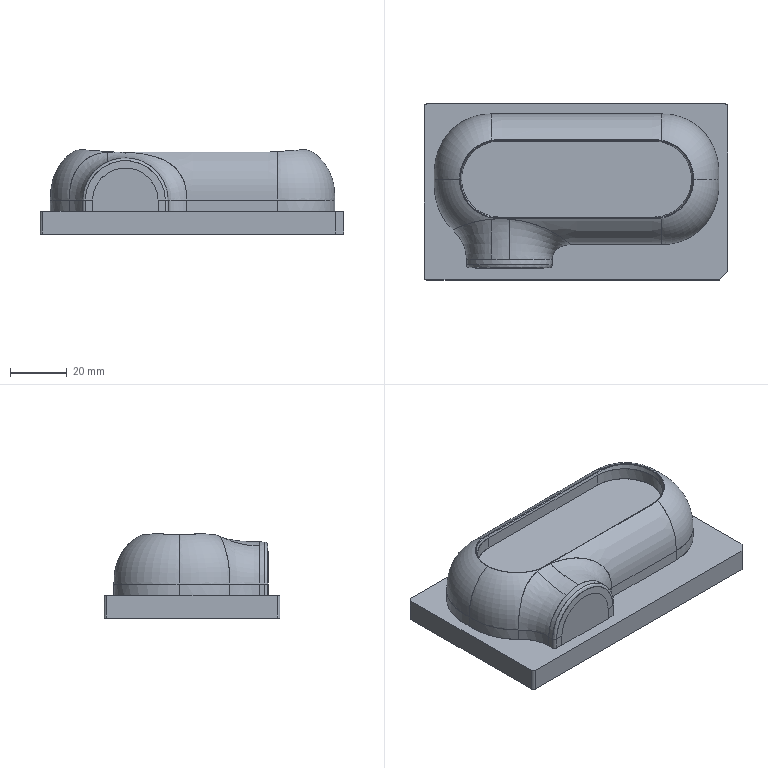NC program | PowerMill | posted by the shop | part box 107 x 62 x 29.663 mm
Lines 35411 to 36775 of 415021:
( TOOL ID   R3_j01_1_1 )
( TOOL DIA. 6. TIP RAD 3. LENGTH 75.84 )
( Z = -20.87 )
T17 M6
T14
G91 G28 Z0
G0 G90 G54
M08
S18000 M3
X0 Y0 M8
G43 Z10.802 H17
X-46.573 Y-.313
Z-2.752
G1 Z-3.952 F1500
X-46.555 Y-.274 Z-3.975 F2500
X-46.539 Y-.233 Z-3.997
X-46.526 Y-.19 Z-4.016
X-46.515 Y-.145 Z-4.032
X-46.507 Y-.099 Z-4.046
X-46.502 Y-.052 Z-4.058
X-46.5 Y-.004 Z-4.067
X-46.501 Y.045 Z-4.073
X-46.504 Y.094 Z-4.076
X-46.508 Y.124
X-46.538 Y.346
X-46.57 Y.607
X-46.602 Y.891
X-46.629 Y1.176
X-46.653 Y1.464
X-46.673 Y1.754
X-46.688 Y2.007
X-46.699 Y2.261
X-46.708 Y2.514
X-46.713 Y2.768
X-46.715 Y3.022
X-46.716 Y3.276
Y3.53
X-46.715 Y4.755
X-46.716 Y5.868
X-46.714 Y6.165
X-46.708 Y6.461
X-46.698 Y6.757
X-46.685 Y7.051
X-46.667 Y7.345
X-46.648 Y7.602
X-46.626 Y7.86
X-46.601 Y8.117
X-46.573 Y8.374
X-46.541 Y8.63
X-46.509 Y8.865
X-46.504 Y8.914 Z-4.075
X-46.502 Y8.963 Z-4.071
Y9.011 Z-4.064
X-46.505 Y9.059 Z-4.054
X-46.512 Y9.106 Z-4.041
X-46.52 Y9.152 Z-4.026
X-46.532 Y9.196 Z-4.009
X-46.546 Y9.238 Z-3.989
X-46.563 Y9.278 Z-3.967
X-46.575 Y9.303 Z-3.952
X-45.957 Y12.216 Z-4.032
X-45.944 Y12.175 Z-4.055
X-45.935 Y12.132 Z-4.077
X-45.928 Y12.087 Z-4.096
X-45.924 Y12.041 Z-4.112
X-45.923 Y11.994 Z-4.126
X-45.925 Y11.947 Z-4.138
X-45.93 Y11.899 Z-4.147
X-45.938 Y11.851 Z-4.153
X-45.948 Y11.803 Z-4.156
X-45.956 Y11.774
X-46.028 Y11.528
X-46.097 Y11.281
X-46.162 Y11.033
X-46.224 Y10.785
X-46.283 Y10.535
X-46.344 Y10.261
X-46.4 Y9.984
X-46.453 Y9.707
X-46.503 Y9.428
X-46.548 Y9.148
X-46.589 Y8.87
X-46.626 Y8.589
X-46.66 Y8.308
X-46.69 Y8.027
X-46.716 Y7.745
X-46.738 Y7.463
X-46.757 Y7.178
X-46.772 Y6.893
X-46.783 Y6.605
X-46.79 Y6.32
X-46.794 Y6.034
Y5.749
Y3.04
X-46.792 Y2.769
X-46.786 Y2.498
X-46.777 Y2.228
X-46.764 Y1.957
X-46.748 Y1.687
X-46.729 Y1.416
X-46.706 Y1.14
X-46.678 Y.86
X-46.647 Y.576
X-46.61 Y.288
X-46.571 Y.006
X-46.528 Y-.272
X-46.482 Y-.546
X-46.433 Y-.817
X-46.378 Y-1.095
X-46.32 Y-1.369
X-46.258 Y-1.641
X-46.194 Y-1.908
X-46.126 Y-2.174
X-46.053 Y-2.44
X-45.977 Y-2.705
X-45.955 Y-2.778
X-45.942 Y-2.826 Z-4.155
X-45.932 Y-2.873 Z-4.151
X-45.926 Y-2.921 Z-4.144
X-45.921 Y-2.969 Z-4.134
X-45.92 Y-3.016 Z-4.122
X-45.922 Y-3.063 Z-4.107
X-45.927 Y-3.109 Z-4.089
X-45.935 Y-3.153 Z-4.069
X-45.945 Y-3.195 Z-4.047
X-45.953 Y-3.221 Z-4.032
X-45.057 Y-5.656 Z-4.112
X-45.051 Y-5.613 Z-4.135
X-45.047 Y-5.569 Z-4.157
Y-5.524 Z-4.176
X-45.049 Y-5.478 Z-4.192
X-45.055 Y-5.432 Z-4.206
X-45.064 Y-5.385 Z-4.218
X-45.075 Y-5.338 Z-4.227
X-45.09 Y-5.292 Z-4.232
X-45.107 Y-5.246 Z-4.236
X-45.119 Y-5.218
X-45.222 Y-4.99
X-45.322 Y-4.761
X-45.42 Y-4.528
X-45.518 Y-4.284
X-45.608 Y-4.051
X-45.695 Y-3.817
X-45.778 Y-3.584
X-45.857 Y-3.35
X-45.934 Y-3.115
X-46.008 Y-2.879
X-46.086 Y-2.615
X-46.161 Y-2.349
X-46.231 Y-2.083
X-46.299 Y-1.813
X-46.362 Y-1.542
X-46.423 Y-1.268
X-46.478 Y-.999
X-46.529 Y-.73
X-46.577 Y-.46
X-46.622 Y-.18
X-46.664 Y.103
X-46.701 Y.376
X-46.734 Y.648
X-46.761 Y.892
X-46.784 Y1.136
X-46.804 Y1.38
X-46.823 Y1.624
X-46.838 Y1.869
X-46.851 Y2.135
X-46.861 Y2.401
X-46.868 Y2.667
X-46.871 Y2.934
X-46.872 Y3.2
Y4.545
X-46.871 Y6.009
X-46.869 Y6.258
X-46.864 Y6.506
X-46.856 Y6.755
X-46.844 Y7.003
X-46.83 Y7.251
X-46.811 Y7.542
X-46.787 Y7.833
X-46.759 Y8.121
X-46.728 Y8.408
X-46.692 Y8.693
X-46.653 Y8.977
X-46.615 Y9.23
X-46.573 Y9.481
X-46.529 Y9.733
X-46.481 Y9.984
X-46.43 Y10.234
X-46.376 Y10.483
X-46.312 Y10.759
X-46.246 Y11.025
X-46.177 Y11.288
X-46.104 Y11.553
X-46.026 Y11.817
X-45.945 Y12.08
X-45.861 Y12.34
X-45.772 Y12.599
X-45.681 Y12.856
X-45.585 Y13.111
X-45.487 Y13.362
X-45.385 Y13.611
X-45.281 Y13.857
X-45.173 Y14.1
X-45.122 Y14.213
X-45.103 Y14.258 Z-4.235
X-45.086 Y14.304 Z-4.231
X-45.073 Y14.351 Z-4.224
X-45.062 Y14.397 Z-4.214
X-45.054 Y14.444 Z-4.202
X-45.05 Y14.49 Z-4.187
X-45.048 Y14.536 Z-4.169
X-45.05 Y14.581 Z-4.149
X-45.054 Y14.624 Z-4.127
X-45.059 Y14.651 Z-4.112
X-43.97 Y16.709 Z-4.192
X-43.969 Y16.666 Z-4.215
X-43.971 Y16.622 Z-4.237
X-43.977 Y16.577 Z-4.256
X-43.986 Y16.532 Z-4.272
X-43.997 Y16.487 Z-4.286
X-44.012 Y16.441 Z-4.298
X-44.03 Y16.397 Z-4.306
X-44.05 Y16.353 Z-4.312
X-44.074 Y16.31 Z-4.316
X-44.089 Y16.283
X-44.194 Y16.115
X-44.297 Y15.946
X-44.398 Y15.775
X-44.497 Y15.604
X-44.594 Y15.431
X-44.71 Y15.218
X-44.823 Y15.004
X-44.933 Y14.788
X-45.041 Y14.571
X-45.145 Y14.352
X-45.258 Y14.106
X-45.367 Y13.858
X-45.472 Y13.61
X-45.573 Y13.361
X-45.67 Y13.111
X-45.761 Y12.865
X-45.85 Y12.617
X-45.934 Y12.369
X-46.015 Y12.119
X-46.093 Y11.868
X-46.167 Y11.616
X-46.241 Y11.352
X-46.311 Y11.085
X-46.379 Y10.815
X-46.443 Y10.542
X-46.501 Y10.274
X-46.557 Y10.003
X-46.609 Y9.727
X-46.658 Y9.447
X-46.703 Y9.165
X-46.745 Y8.881
X-46.783 Y8.596
X-46.816 Y8.312
X-46.846 Y8.029
X-46.872 Y7.74
X-46.895 Y7.449
X-46.914 Y7.156
X-46.928 Y6.861
X-46.939 Y6.564
X-46.946 Y6.266
X-46.949 Y5.966
Y5.664
Y3.939
Y3.606
Y3.365
Y3.124
X-46.948 Y2.883
X-46.944 Y2.642
X-46.938 Y2.402
X-46.929 Y2.161
X-46.915 Y1.876
X-46.898 Y1.591
X-46.876 Y1.307
X-46.851 Y1.02
X-46.822 Y.734
X-46.788 Y.449
X-46.751 Y.165
X-46.714 Y-.095
X-46.673 Y-.355
X-46.629 Y-.614
X-46.582 Y-.872
X-46.531 Y-1.13
X-46.473 Y-1.403
X-46.412 Y-1.675
X-46.349 Y-1.937
X-46.282 Y-2.199
X-46.209 Y-2.47
X-46.147 Y-2.686
X-46.083 Y-2.902
X-46.016 Y-3.117
X-45.947 Y-3.331
X-45.859 Y-3.591
X-45.767 Y-3.849
X-45.672 Y-4.104
X-45.574 Y-4.357
X-45.473 Y-4.607
X-45.368 Y-4.855
X-45.26 Y-5.1
X-45.149 Y-5.343
X-45.035 Y-5.583
X-44.917 Y-5.822
X-44.795 Y-6.058
X-44.67 Y-6.292
X-44.542 Y-6.524
X-44.411 Y-6.753
X-44.277 Y-6.98
X-44.139 Y-7.205
X-44.088 Y-7.287
X-44.063 Y-7.329 Z-4.315
X-44.041 Y-7.372 Z-4.311
X-44.021 Y-7.417 Z-4.304
X-44.004 Y-7.462 Z-4.294
X-43.991 Y-7.507 Z-4.281
X-43.98 Y-7.552 Z-4.266
X-43.972 Y-7.597 Z-4.249
X-43.968 Y-7.642 Z-4.229
X-43.967 Y-7.686 Z-4.207
Y-7.712 Z-4.192
X-42.694 Y-9.513 Z-4.272
X-42.699 Y-9.471 Z-4.295
X-42.706 Y-9.427 Z-4.317
X-42.718 Y-9.384 Z-4.336
X-42.732 Y-9.34 Z-4.352
X-42.749 Y-9.296 Z-4.366
X-42.77 Y-9.253 Z-4.378
X-42.793 Y-9.211 Z-4.386
X-42.819 Y-9.17 Z-4.392
X-42.847 Y-9.13 Z-4.396
X-42.866 Y-9.106
X-43.03 Y-8.906
X-43.191 Y-8.702
X-43.349 Y-8.496
X-43.504 Y-8.287
X-43.656 Y-8.076
X-43.804 Y-7.862
X-43.95 Y-7.645
X-44.093 Y-7.426
X-44.233 Y-7.204
X-44.369 Y-6.98
X-44.503 Y-6.752
X-44.634 Y-6.522
X-44.762 Y-6.289
X-44.886 Y-6.054
X-45.007 Y-5.816
X-45.124 Y-5.579
X-45.237 Y-5.34
X-45.347 Y-5.099
X-45.453 Y-4.855
X-45.556 Y-4.611
X-45.643 Y-4.395
X-45.728 Y-4.178
X-45.81 Y-3.961
X-45.888 Y-3.742
X-45.965 Y-3.522
X-46.05 Y-3.266
X-46.132 Y-3.007
X-46.211 Y-2.745
X-46.286 Y-2.48
X-46.359 Y-2.211
X-46.428 Y-1.939
X-46.494 Y-1.664
X-46.551 Y-1.412
X-46.604 Y-1.16
X-46.654 Y-.907
X-46.701 Y-.653
X-46.744 Y-.398
X-46.788 Y-.122
X-46.826 Y.143
X-46.862 Y.419
X-46.895 Y.696
X-46.924 Y.973
X-46.949 Y1.252
X-46.97 Y1.53
X-46.988 Y1.808
X-47.002 Y2.071
X-47.012 Y2.334
X-47.02 Y2.597
X-47.024 Y2.861
X-47.025 Y3.124
Y3.387
Y5.574
Y5.868
X-47.024 Y6.154
X-47.019 Y6.44
X-47.01 Y6.726
X-46.999 Y6.999
X-46.984 Y7.267
X-46.965 Y7.534
X-46.944 Y7.801
X-46.919 Y8.074
X-46.891 Y8.34
X-46.859 Y8.606
X-46.824 Y8.872
X-46.784 Y9.143
X-46.742 Y9.414
X-46.694 Y9.689
X-46.643 Y9.965
X-46.588 Y10.236
X-46.53 Y10.504
X-46.468 Y10.771
X-46.403 Y11.038
X-46.335 Y11.3
X-46.263 Y11.562
X-46.188 Y11.822
X-46.108 Y12.084
X-46.025 Y12.342
X-45.938 Y12.599
X-45.853 Y12.84
X-45.765 Y13.08
X-45.673 Y13.319
X-45.578 Y13.557
X-45.479 Y13.793
X-45.378 Y14.028
X-45.268 Y14.273
X-45.154 Y14.515
X-45.038 Y14.755
X-44.918 Y14.992
X-44.795 Y15.227
X-44.669 Y15.459
X-44.539 Y15.69
X-44.406 Y15.918
X-44.27 Y16.143
X-44.132 Y16.366
X-43.989 Y16.586
X-43.844 Y16.803
X-43.696 Y17.018
X-43.545 Y17.231
X-43.39 Y17.441
X-43.266 Y17.604
X-43.142 Y17.765
X-43.015 Y17.924
X-42.886 Y18.082
X-42.871 Y18.1
X-42.841 Y18.139 Z-4.395
X-42.813 Y18.178 Z-4.391
X-42.788 Y18.22 Z-4.384
X-42.765 Y18.262 Z-4.374
X-42.745 Y18.305 Z-4.361
X-42.728 Y18.349 Z-4.346
X-42.715 Y18.392 Z-4.329
X-42.704 Y18.436 Z-4.309
X-42.697 Y18.479 Z-4.287
X-42.695 Y18.505 Z-4.272
X-41.159 Y20.163 Z-4.352
X-41.169 Y20.122 Z-4.375
X-41.183 Y20.08 Z-4.397
X-41.2 Y20.038 Z-4.416
X-41.22 Y19.997 Z-4.432
X-41.243 Y19.956 Z-4.446
X-41.269 Y19.916 Z-4.458
X-41.298 Y19.877 Z-4.466
X-41.329 Y19.84 Z-4.472
X-41.362 Y19.804 Z-4.476
X-41.385 Y19.783
X-41.568 Y19.612
X-41.749 Y19.437
X-41.93 Y19.257
X-42.109 Y19.073
X-42.288 Y18.885
X-42.457 Y18.7
X-42.624 Y18.513
X-42.788 Y18.322
X-42.95 Y18.13
X-43.106 Y17.938
X-43.259 Y17.743
X-43.41 Y17.546
X-43.565 Y17.338
X-43.709 Y17.137
X-43.851 Y16.933
X-43.99 Y16.728
X-44.133 Y16.508
X-44.274 Y16.286
X-44.412 Y16.061
X-44.547 Y15.834
X-44.678 Y15.604
X-44.806 Y15.372
X-44.931 Y15.137
X-45.052 Y14.9
X-45.17 Y14.661
X-45.285 Y14.42
X-45.397 Y14.177
X-45.503 Y13.936
X-45.607 Y13.689
X-45.708 Y13.441
X-45.806 Y13.19
X-45.9 Y12.939
X-45.989 Y12.686
X-46.076 Y12.433
X-46.161 Y12.17
X-46.243 Y11.905
X-46.321 Y11.639
X-46.396 Y11.371
X-46.466 Y11.102
X-46.533 Y10.832
X-46.595 Y10.563
X-46.655 Y10.29
X-46.711 Y10.012
X-46.763 Y9.734
X-46.811 Y9.459
X-46.855 Y9.184
X-46.896 Y8.901
X-46.934 Y8.615
X-46.968 Y8.326
X-46.999 Y8.033
X-47.025 Y7.75
X-47.045 Y7.482
X-47.062 Y7.216
X-47.076 Y6.945
X-47.087 Y6.674
X-47.095 Y6.403
X-47.099 Y6.131
X-47.101 Y5.86
Y5.588
X-47.099 Y4.305
X-47.1 Y3.394
Y3.14
X-47.099 Y2.824
X-47.094 Y2.559
X-47.087 Y2.306
X-47.074 Y2.009
X-47.058 Y1.721
X-47.04 Y1.45
X-47.018 Y1.18
X-46.993 Y.91
X-46.965 Y.641
X-46.933 Y.372
X-46.895 Y.085
X-46.853 Y-.2
X-46.807 Y-.483
X-46.758 Y-.764
X-46.705 Y-1.042
X-46.649 Y-1.318
X-46.591 Y-1.581
X-46.531 Y-1.842
X-46.466 Y-2.101
X-46.398 Y-2.36
X-46.327 Y-2.618
X-46.254 Y-2.868
X-46.178 Y-3.117
X-46.099 Y-3.365
X-46.016 Y-3.611
X-45.931 Y-3.852
X-45.843 Y-4.091
X-45.753 Y-4.329
X-45.658 Y-4.566
X-45.561 Y-4.801
X-45.46 Y-5.035
X-45.355 Y-5.267
X-45.248 Y-5.499
X-45.136 Y-5.731
X-45.021 Y-5.963
X-44.901 Y-6.194
X-44.779 Y-6.421
X-44.653 Y-6.647
X-44.525 Y-6.871
X-44.391 Y-7.096
X-44.254 Y-7.319
X-44.112 Y-7.541
X-43.968 Y-7.761
X-43.82 Y-7.978
X-43.67 Y-8.192
X-43.521 Y-8.397
X-43.37 Y-8.599
X-43.214 Y-8.801
X-43.052 Y-9.004
X-42.887 Y-9.206
X-42.718 Y-9.405
X-42.548 Y-9.599
X-42.377 Y-9.788
X-42.205 Y-9.973
X-42.053 Y-10.132
X-41.898 Y-10.289
X-41.742 Y-10.444
X-41.583 Y-10.597
X-41.422 Y-10.748
X-41.398 Y-10.771
X-41.363 Y-10.805 Z-4.475
X-41.33 Y-10.841 Z-4.471
X-41.299 Y-10.879 Z-4.464
X-41.271 Y-10.918 Z-4.454
X-41.246 Y-10.958 Z-4.441
X-41.224 Y-10.999 Z-4.426
X-41.205 Y-11.04 Z-4.409
X-41.189 Y-11.082 Z-4.389
X-41.176 Y-11.124 Z-4.367
X-41.17 Y-11.15 Z-4.352
X-39.452 Y-12.568 Z-4.432
X-39.468 Y-12.528 Z-4.455
X-39.487 Y-12.489 Z-4.477
X-39.509 Y-12.449 Z-4.496
X-39.535 Y-12.411 Z-4.512
X-39.563 Y-12.374 Z-4.526
X-39.594 Y-12.338 Z-4.538
X-39.628 Y-12.303 Z-4.546
X-39.663 Y-12.27 Z-4.552
X-39.701 Y-12.239 Z-4.556
X-39.726 Y-12.221
X-39.928 Y-12.077
X-40.131 Y-11.929
X-40.333 Y-11.775
X-40.535 Y-11.616
X-40.734 Y-11.455
X-40.929 Y-11.292
X-41.119 Y-11.128
X-41.307 Y-10.962
X-41.492 Y-10.792
X-41.675 Y-10.62
X-41.857 Y-10.442
X-42.034 Y-10.264
X-42.209 Y-10.084
X-42.381 Y-9.901
X-42.55 Y-9.715
X-42.722 Y-9.521
X-42.89 Y-9.324
X-43.052 Y-9.129
X-43.211 Y-8.932
X-43.367 Y-8.732
X-43.522 Y-8.527
X-43.676 Y-8.317
X-43.826 Y-8.106
X-43.97 Y-7.898
X-44.11 Y-7.687
X-44.25 Y-7.47
X-44.386 Y-7.252
X-44.52 Y-7.031
X-44.652 Y-6.806
X-44.779 Y-6.582
X-44.902 Y-6.356
X-45.022 Y-6.128
X-45.135 Y-5.906
X-45.246 Y-5.683
X-45.353 Y-5.458
X-45.457 Y-5.231
X-45.557 Y-5.004
X-45.655 Y-4.774
X-45.749 Y-4.544
X-45.847 Y-4.295
X-45.943 Y-4.042
X-46.036 Y-3.783
X-46.127 Y-3.518
X-46.211 Y-3.263
X-46.293 Y-3.003
X-46.372 Y-2.738
X-46.448 Y-2.467
X-46.515 Y-2.214
X-46.58 Y-1.961
X-46.641 Y-1.704
X-46.698 Y-1.448
X-46.752 Y-1.193
X-46.802 Y-.937
X-46.849 Y-.681
X-46.893 Y-.424
X-46.934 Y-.166
X-46.974 Y.113
X-47.011 Y.393
X-47.044 Y.673
X-47.073 Y.956
X-47.098 Y1.237
X-47.12 Y1.518
X-47.137 Y1.787
X-47.152 Y2.056
X-47.162 Y2.325
X-47.17 Y2.594
X-47.174 Y2.864
Y3.133
X-47.175 Y5.585
Y5.825
X-47.174 Y6.066
X-47.171 Y6.306
X-47.166 Y6.546
X-47.158 Y6.786
X-47.145 Y7.072
X-47.128 Y7.358
X-47.108 Y7.644
X-47.084 Y7.929
X-47.055 Y8.218
X-47.023 Y8.506
X-46.987 Y8.794
X-46.947 Y9.08
X-46.902 Y9.367
X-46.855 Y9.647
X-46.804 Y9.926
X-46.749 Y10.204
X-46.691 Y10.482
X-46.629 Y10.755
X-46.563 Y11.026
X-46.494 Y11.297
X-46.42 Y11.566
X-46.343 Y11.834
X-46.262 Y12.101
X-46.178 Y12.367
X-46.097 Y12.607
X-46.014 Y12.846
X-45.927 Y13.084
X-45.837 Y13.321
X-45.744 Y13.557
X-45.641 Y13.807
X-45.534 Y14.056
X-45.424 Y14.303
X-45.31 Y14.548
X-45.193 Y14.79
X-45.073 Y15.03
X-44.95 Y15.267
X-44.824 Y15.5
X-44.695 Y15.731
X-44.567 Y15.952
X-44.434 Y16.175
X-44.295 Y16.398
X-44.153 Y16.621
X-44.008 Y16.841
X-43.862 Y17.055
X-43.715 Y17.263
X-43.568 Y17.465
X-43.417 Y17.666
X-43.264 Y17.864
X-43.109 Y18.059
X-42.95 Y18.253
X-42.788 Y18.444
X-42.623 Y18.632
X-42.456 Y18.818
X-42.282 Y19.006
X-42.105 Y19.191
X-41.926 Y19.374
X-41.743 Y19.553
X-41.56 Y19.729
X-41.373 Y19.901
X-41.181 Y20.074
X-40.99 Y20.241
X-40.796 Y20.405
X-40.633 Y20.538
X-40.468 Y20.669
X-40.302 Y20.798
X-40.129 Y20.929
X-39.96 Y21.054
X-39.789 Y21.177
X-39.726 Y21.221
X-39.687 Y21.25 Z-4.555
X-39.65 Y21.281 Z-4.55
X-39.614 Y21.315 Z-4.544
X-39.582 Y21.349 Z-4.534
X-39.551 Y21.386 Z-4.521
X-39.524 Y21.424 Z-4.506
X-39.499 Y21.462 Z-4.489
X-39.478 Y21.501 Z-4.469
X-39.46 Y21.541 Z-4.447
X-39.45 Y21.566 Z-4.432
X-37.168 Y22.926 Z-4.512
X-37.19 Y22.889 Z-4.535
X-37.215 Y22.853 Z-4.557
X-37.243 Y22.818 Z-4.576
X-37.274 Y22.784 Z-4.592
X-37.308 Y22.751 Z-4.606
X-37.345 Y22.721 Z-4.618
X-37.383 Y22.692 Z-4.626
X-37.424 Y22.665 Z-4.632
X-37.466 Y22.641 Z-4.636
X-37.493 Y22.627
X-37.715 Y22.517
X-37.935 Y22.404
X-38.159 Y22.285
X-38.383 Y22.161
X-38.599 Y22.038
X-38.811 Y21.912
X-39.022 Y21.782
X-39.239 Y21.645
X-39.453 Y21.504
X-39.666 Y21.36
X-39.876 Y21.213
X-40.084 Y21.062
X-40.289 Y20.908
X-40.493 Y20.75
X-40.686 Y20.596
X-40.878 Y20.438
X-41.067 Y20.278
X-41.261 Y20.109
X-41.445 Y19.943
X-41.626 Y19.774
X-41.805 Y19.602
X-41.983 Y19.427
X-42.159 Y19.249
X-42.333 Y19.067
X-42.503 Y18.883
X-42.67 Y18.697
X-42.823 Y18.522
X-42.974 Y18.345
X-43.122 Y18.166
X-43.268 Y17.984
X-43.427 Y17.78
X-43.584 Y17.573
X-43.738 Y17.364
X-43.889 Y17.151
X-44.037 Y16.935
X-44.182 Y16.717
X-44.324 Y16.497
X-44.463 Y16.274
X-44.598 Y16.049
X-44.732 Y15.819
X-44.863 Y15.587
X-44.99 Y15.353
X-45.114 Y15.116
X-45.235 Y14.877
X-45.353 Y14.635
X-45.467 Y14.392
X-45.578 Y14.145
X-45.685 Y13.897
X-45.79 Y13.645
X-45.891 Y13.391
X-45.989 Y13.135
X-46.083 Y12.878
X-46.173 Y12.618
X-46.26 Y12.357
X-46.344 Y12.093
X-46.424 Y11.826
X-46.501 Y11.558
X-46.573 Y11.289
X-46.642 Y11.018
X-46.708 Y10.745
X-46.77 Y10.47
X-46.828 Y10.192
X-46.883 Y9.913
X-46.933 Y9.633
X-46.98 Y9.351
X-47.024 Y9.066
X-47.064 Y8.779
X-47.099 Y8.499
X-47.13 Y8.218
X-47.158 Y7.938
X-47.181 Y7.656
X-47.201 Y7.374
X-47.218 Y7.093
X-47.231 Y6.815
X-47.24 Y6.537
X-47.246 Y6.258
X-47.248 Y5.98
X-47.249 Y5.702
X-47.248 Y4.351
X-47.249 Y3.181
X-47.248 Y2.893
X-47.243 Y2.6
X-47.235 Y2.302
X-47.223 Y2.005
X-47.207 Y1.715
X-47.188 Y1.426
X-47.164 Y1.139
X-47.138 Y.857
X-47.107 Y.573
X-47.072 Y.289
X-47.034 Y.004
X-46.992 Y-.28
X-46.946 Y-.562
X-46.896 Y-.841
X-46.843 Y-1.118
X-46.786 Y-1.395
X-46.727 Y-1.661
X-46.665 Y-1.927
X-46.597 Y-2.197
X-46.524 Y-2.472
X-46.45 Y-2.738
X-46.371 Y-3.003
X-46.289 Y-3.267
X-46.203 Y-3.531
X-46.113 Y-3.793
X-46.023 Y-4.043
X-45.93 Y-4.291
X-45.833 Y-4.538
X-45.733 Y-4.783
X-45.629 Y-5.027
X-45.521 Y-5.273
X-45.408 Y-5.517
X-45.293 Y-5.759
X-45.174 Y-5.999
X-45.051 Y-6.237
X-44.926 Y-6.473
X-44.797 Y-6.706
X-44.67 Y-6.926
X-44.541 Y-7.145
X-44.409 Y-7.361
X-44.274 Y-7.576
X-44.135 Y-7.789
X-43.993 Y-7.999
X-43.849 Y-8.208
X-43.701 Y-8.414
X-43.549 Y-8.62
X-43.391 Y-8.827
X-43.233 Y-9.028
X-43.071 Y-9.228
X-42.904 Y-9.427
X-42.734 Y-9.624
X-42.562 Y-9.818
X-42.389 Y-10.007
X-42.212 Y-10.194
X-42.031 Y-10.379
X-41.846 Y-10.562
X-41.66 Y-10.742
X-41.473 Y-10.917
X-41.283 Y-11.088
X-41.091 Y-11.257
X-40.895 Y-11.424
X-40.695 Y-11.589
X-40.508 Y-11.739
X-40.318 Y-11.886
X-40.127 Y-12.03
X-39.933 Y-12.171
X-39.734 Y-12.312
X-39.533 Y-12.451
X-39.33 Y-12.586
X-39.125 Y-12.718
X-38.918 Y-12.847
X-38.709 Y-12.973
X-38.661 Y-13.002
X-38.62 Y-13.028 Z-4.635
X-38.58 Y-13.056 Z-4.63
X-38.543 Y-13.087 Z-4.623
X-38.507 Y-13.119 Z-4.614
X-38.475 Y-13.153 Z-4.601
X-38.444 Y-13.189 Z-4.586
X-38.417 Y-13.225 Z-4.569
X-38.393 Y-13.263 Z-4.549
X-38.372 Y-13.301 Z-4.527
X-38.36 Y-13.326 Z-4.512
X-38.263 Y-13.48 Z-4.592
X-38.281 Y-13.441 Z-4.615
X-38.303 Y-13.403 Z-4.637
X-38.329 Y-13.365 Z-4.656
X-38.357 Y-13.329 Z-4.672
X-38.388 Y-13.294 Z-4.686
X-38.422 Y-13.26 Z-4.698
X-38.458 Y-13.228 Z-4.706
X-38.496 Y-13.198 Z-4.712
X-38.536 Y-13.171 Z-4.715
X-38.562 Y-13.154 Z-4.716
X-38.755 Y-13.038
X-38.946 Y-12.922
X-39.137 Y-12.803
X-39.326 Y-12.682
X-39.514 Y-12.558
X-39.72 Y-12.418
X-39.927 Y-12.272
X-40.137 Y-12.12
X-40.338 Y-11.969
X-40.536 Y-11.816
X-40.731 Y-11.66
X-40.928 Y-11.498
X-41.123 Y-11.333
X-41.315 Y-11.164
X-41.506 Y-10.992
X-41.694 Y-10.816
X-41.88 Y-10.637
X-42.063 Y-10.456
X-42.243 Y-10.273
X-42.41 Y-10.097
X-42.574 Y-9.919
X-42.736 Y-9.738
X-42.903 Y-9.547
X-43.059 Y-9.362
X-43.214 Y-9.175
X-43.371 Y-8.977
X-43.525 Y-8.778
X-43.679 Y-8.574
X-43.833 Y-8.361
X-43.984 Y-8.147
X-44.127 Y-7.938
X-44.266 Y-7.728
X-44.402 Y-7.515
X-44.543 Y-7.288
X-44.681 Y-7.059
X-44.815 Y-6.827
X-44.946 Y-6.594
X-45.073 Y-6.358
X-45.197 Y-6.12
X-45.317 Y-5.881
X-45.434 Y-5.639
X-45.548 Y-5.395
X-45.656 Y-5.153
X-45.761 Y-4.909
X-45.863 Y-4.664
X-45.961 Y-4.418
X-46.057 Y-4.166
X-46.148 Y-3.917
X-46.235 Y-3.667
X-46.319 Y-3.415
X-46.4 Y-3.163
X-46.479 Y-2.902
X-46.555 Y-2.64
X-46.628 Y-2.374
X-46.696 Y-2.11
X-46.76 Y-1.845
X-46.821 Y-1.579
X-46.88 Y-1.304
X-46.936 Y-1.028
X-46.988 Y-.75
X-47.036 Y-.469
X-47.08 Y-.187
X-47.121 Y.095
X-47.157 Y.376
X-47.19 Y.655
X-47.219 Y.935
X-47.244 Y1.215
X-47.266 Y1.495
X-47.283 Y1.768
X-47.298 Y2.039
X-47.309 Y2.311
X-47.316 Y2.583
X-47.32 Y2.855
X-47.321 Y3.127
Y5.444
Y5.674
Y5.903
X-47.32 Y6.133
X-47.317 Y6.362
X-47.312 Y6.592
X-47.304 Y6.821
X-47.293 Y7.051
X-47.277 Y7.339
X-47.257 Y7.629
X-47.232 Y7.921
X-47.204 Y8.212
X-47.172 Y8.5
X-47.137 Y8.786
X-47.097 Y9.073
X-47.059 Y9.327
X-47.017 Y9.582
X-46.972 Y9.836
X-46.924 Y10.089
X-46.873 Y10.342
X-46.813 Y10.616
X-46.749 Y10.891
X-46.682 Y11.163
X-46.613 Y11.429
X-46.545 Y11.675
X-46.474 Y11.92
X-46.4 Y12.164
X-46.322 Y12.407
X-46.241 Y12.649
X-46.152 Y12.906
X-46.058 Y13.162
X-45.961 Y13.418
X-45.86 Y13.671
X-45.756 Y13.921
X-45.649 Y14.169
X-45.538 Y14.416
X-45.428 Y14.651
X-45.315 Y14.884
X-45.199 Y15.116
X-45.079 Y15.347
X-44.955 Y15.575
X-44.828 Y15.803
X-44.697 Y16.031
X-44.562 Y16.257
X-44.424 Y16.481
X-44.284 Y16.701
X-44.141 Y16.918
X-43.994 Y17.132
X-43.845 Y17.345
X-43.691 Y17.557
X-43.535 Y17.766
X-43.375 Y17.973
X-43.211 Y18.177
X-43.045 Y18.379
X-42.876 Y18.579
X-42.704 Y18.775
X-42.529 Y18.968
X-42.352 Y19.158
X-42.173 Y19.345
X-41.991 Y19.529
X-41.806 Y19.71
X-41.618 Y19.888
X-41.428 Y20.063
X-41.235 Y20.235
X-41.04 Y20.404
X-40.842 Y20.57
X-40.642 Y20.732
X-40.441 Y20.89
X-40.236 Y21.046
X-40.029 Y21.199
X-39.819 Y21.349
X-39.607 Y21.495
X-39.392 Y21.639
X-39.175 Y21.779
X-38.956 Y21.916
X-38.735 Y22.049
X-38.513 Y22.178
X-38.288 Y22.304
X-38.062 Y22.427
X-37.836 Y22.545
X-37.608 Y22.659
X-37.379 Y22.77
X-37.146 Y22.878
X-36.913 Y22.982
X-36.679 Y23.082
X-36.443 Y23.179
X-36.203 Y23.274
X-35.961 Y23.364
X-35.717 Y23.452
X-35.472 Y23.535
X-35.225 Y23.615
X-34.976 Y23.692
X-34.737 Y23.762
X-34.516 Y23.823
X-34.365 Y23.862
X-34.318 Y23.876 Z-4.715
X-34.272 Y23.892 Z-4.71
X-34.228 Y23.911 Z-4.703
X-34.185 Y23.932 Z-4.694
X-34.144 Y23.956 Z-4.681
X-34.105 Y23.982 Z-4.666
X-34.068 Y24.009 Z-4.649
X-34.035 Y24.039 Z-4.629
X-34.004 Y24.07 Z-4.607
X-33.986 Y24.09 Z-4.592
G0 Z2.966
G1 X47.016 Y9.304 F10000
G0 Z-2.752
G1 Z-3.952 F1500
X46.997 Y9.265 Z-3.976 F2500
X46.981 Y9.224 Z-3.997
X46.968 Y9.181 Z-4.016
X46.957 Y9.136 Z-4.032
X46.949 Y9.09 Z-4.046
X46.944 Y9.043 Z-4.058
X46.942 Y8.995 Z-4.067
Y8.946 Z-4.073
X46.946 Y8.897 Z-4.076
X46.949 Y8.867
X46.984 Y8.607
X47.016 Y8.346
X47.045 Y8.085
X47.069 Y7.824
X47.091 Y7.563
X47.112 Y7.275
X47.128 Y6.986
X47.141 Y6.695
X47.15 Y6.403
X47.155 Y6.109
X47.156 Y5.813
X47.155 Y4.171
X47.156 Y3.181
X47.155 Y2.872
X47.15 Y2.591
X47.141 Y2.305
X47.128 Y2.01
X47.113 Y1.743
X47.095 Y1.478
X47.073 Y1.212
X47.046 Y.93
X47.017 Y.665
X46.985 Y.4
X46.949 Y.136
Y.13
X46.943 Y.082 Z-4.075
X46.94 Y.033 Z-4.071
X46.941 Y-.016 Z-4.064
X46.944 Y-.063 Z-4.054
X46.949 Y-.11 Z-4.041
X46.958 Y-.156 Z-4.026
X46.969 Y-.2 Z-4.009
X46.983 Y-.243 Z-3.989
X47. Y-.283 Z-3.967
X47.012 Y-.307 Z-3.952
X46.397 Y-3.214 Z-4.032
X46.384 Y-3.173 Z-4.055
X46.375 Y-3.13 Z-4.077
X46.368 Y-3.086 Z-4.096
X46.364 Y-3.04 Z-4.112
X46.363 Y-2.993 Z-4.126
X46.365 Y-2.945 Z-4.138
X46.37 Y-2.897 Z-4.147
X46.378 Y-2.85 Z-4.153
X46.389 Y-2.802 Z-4.156
X46.397 Y-2.772
X46.467 Y-2.535
X46.536 Y-2.284
X46.599 Y-2.044
X46.665 Y-1.782
X46.727 Y-1.519
X46.785 Y-1.256
X46.84 Y-.988
X46.891 Y-.723
X46.938 Y-.457
X46.981 Y-.191
X47.021 Y.076
X47.059 Y.352
X47.094 Y.634
X47.125 Y.92
X47.151 Y1.204
X47.174 Y1.483
X47.194 Y1.776
X47.21 Y2.07
X47.222 Y2.364
X47.23 Y2.658
X47.234 Y2.953
X47.235 Y3.249
X47.234 Y3.818
Y5.199
X47.235 Y5.868
X47.233 Y6.168
X47.227 Y6.47
X47.217 Y6.764
X47.204 Y7.057
X47.186 Y7.35
X47.165 Y7.641
X47.139 Y7.93
X47.11 Y8.219
X47.077 Y8.506
X47.044 Y8.763
X47.007 Y9.02
X46.968 Y9.277
X46.923 Y9.544
X46.876 Y9.8
X46.827 Y10.054
X46.773 Y10.309
X46.716 Y10.567
X46.655 Y10.824
X46.59 Y11.08
X46.522 Y11.335
X46.456 Y11.57
X46.398 Y11.767
X46.386 Y11.814 Z-4.155
X46.376 Y11.862 Z-4.151
X46.37 Y11.91 Z-4.144
X46.366 Y11.958 Z-4.134
X46.365 Y12.005 Z-4.121
X46.367 Y12.052 Z-4.106
X46.372 Y12.097 Z-4.089
X46.379 Y12.141 Z-4.069
X46.39 Y12.183 Z-4.047
X46.398 Y12.209 Z-4.032
X45.501 Y14.647 Z-4.112
X45.495 Y14.605 Z-4.135
X45.491 Y14.561 Z-4.157
Y14.516 Z-4.176
X45.494 Y14.47 Z-4.192
X45.499 Y14.424 Z-4.206
X45.508 Y14.377 Z-4.218
X45.519 Y14.33 Z-4.227
X45.534 Y14.284 Z-4.232
X45.551 Y14.238 Z-4.236
X45.563 Y14.21
X45.656 Y14.005
X45.743 Y13.807
X45.821 Y13.622
X45.897 Y13.437
X45.971 Y13.25
X46.044 Y13.063
X46.114 Y12.875
X46.2 Y12.636
X46.282 Y12.396
X46.362 Y12.154
X46.438 Y11.912
X46.51 Y11.669
X46.584 Y11.409
X46.654 Y11.149
X46.721 Y10.885
X46.784 Y10.623
X46.843 Y10.36
X46.896 Y10.109
X46.945 Y9.858
X46.992 Y9.606
X47.035 Y9.354
X47.075 Y9.101
X47.116 Y8.812
X47.154 Y8.523
X47.187 Y8.237
X47.216 Y7.951
X47.241 Y7.666
X47.263 Y7.371
X47.28 Y7.087
X47.294 Y6.802
X47.304 Y6.51
X47.31 Y6.213
X47.312 Y5.908
Y5.595
Y3.04
X47.31 Y2.771
X47.304 Y2.491
X47.294 Y2.197
X47.281 Y1.929
X47.264 Y1.65
X47.243 Y1.366
X47.218 Y1.074
X47.189 Y.787
X47.158 Y.51
X47.123 Y.233
X47.083 Y-.043
X47.04 Y-.324
X46.992 Y-.604
X46.941 Y-.881
X46.886 Y-1.156
X46.828 Y-1.429
X46.766 Y-1.701
X46.699 Y-1.972
X46.634 Y-2.226
X46.565 Y-2.48
X46.492 Y-2.732
X46.416 Y-2.983
X46.335 Y-3.235
X46.249 Y-3.493
X46.161 Y-3.746
X46.07 Y-3.995
X45.984 Y-4.217
X45.896 Y-4.439
X45.804 Y-4.663
X45.71 Y-4.882
X45.613 Y-5.1
X45.56 Y-5.216
X45.541 Y-5.261 Z-4.235
X45.524 Y-5.307 Z-4.231
X45.511 Y-5.354 Z-4.224
X45.5 Y-5.4 Z-4.214
X45.492 Y-5.447 Z-4.201
X45.488 Y-5.494 Z-4.186
X45.486 Y-5.539 Z-4.169
X45.487 Y-5.584 Z-4.149
X45.492 Y-5.627 Z-4.127
X45.496 Y-5.654 Z-4.112
X44.408 Y-7.715 Z-4.192
X44.407 Y-7.672 Z-4.215
X44.409 Y-7.628 Z-4.237
X44.415 Y-7.584 Z-4.256
X44.423 Y-7.538 Z-4.272
X44.435 Y-7.493 Z-4.286
X44.449 Y-7.448 Z-4.298
X44.467 Y-7.403 Z-4.306
X44.487 Y-7.359 Z-4.312
X44.51 Y-7.316 Z-4.316
X44.526 Y-7.289
X44.666 Y-7.064
X44.802 Y-6.836
X44.935 Y-6.607
X45.064 Y-6.376
X45.19 Y-6.144
X45.312 Y-5.909
X45.432 Y-5.671
X45.548 Y-5.431
X45.66 Y-5.189
X45.769 Y-4.944
X45.875 Y-4.698
X45.976 Y-4.453
X46.074 Y-4.206
X46.168 Y-3.958
X46.258 Y-3.708
X46.345 Y-3.456
X46.428 Y-3.204
X46.508 Y-2.951
X46.584 Y-2.697
X46.656 Y-2.442
X46.726 Y-2.186
X46.791 Y-1.929
X46.853 Y-1.672
X46.911 Y-1.413
X46.967 Y-1.152
X47.019 Y-.889
X47.067 Y-.626
X47.112 Y-.362
X47.154 Y-.098
X47.193 Y.176
X47.229 Y.45
X47.262 Y.736
X47.291 Y1.021
X47.316 Y1.296